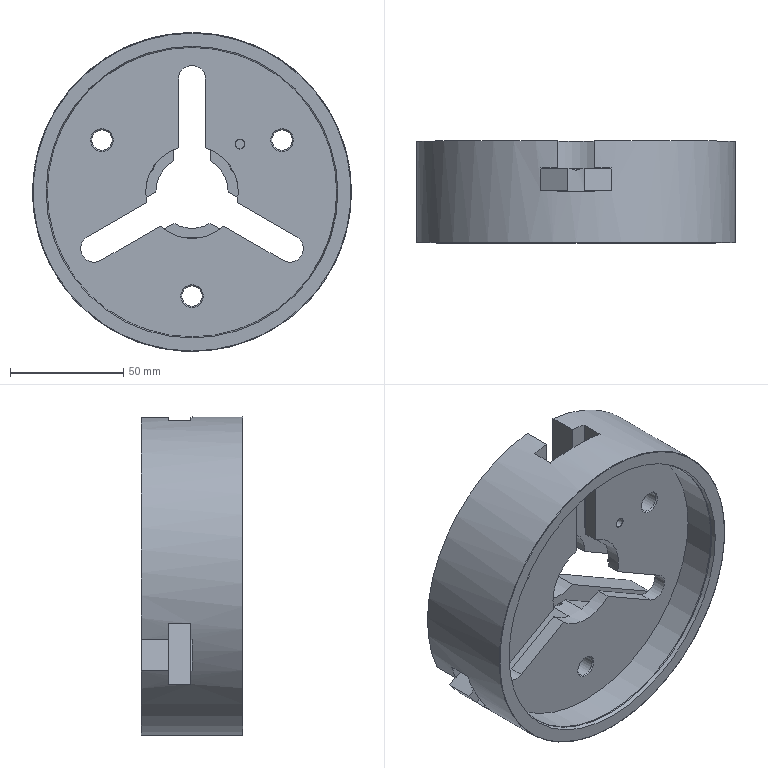NC program | NX | posted with a generic post | part box 141 x 45 x 141 mm
Whole program:
N10 G17 G21 G94 G90
(PLANAR_MILL , TOOL : D14)
N12 T05 M6
N14 G54
N16 G17 G0 G90 X0. Y89. S3600 M3
N18 G43 Z100. H5
N20 Z-1.
N22 G94 G1 Z-2. F3600.
N24 Y75.
N26 X0.9
N28 Y7.1
N30 X-0.9
N32 Y75.
N34 X0.
N36 Y89.
N38 Z-1.
N40 G0 Z0.3
N42 Z-3.
N44 G1 Z-4.
N46 Y75.
N48 X0.9
N50 Y7.1
N52 X-0.9
N54 Y75.
N56 X0.
N58 Y89.
N60 Z-3.
N62 G0 Z-1.7
N64 Z-5.
N66 G1 Z-6.
N68 Y75.
N70 X0.9
N72 Y7.1
N74 X-0.9
N76 Y75.
N78 X0.
N80 Y89.
N82 Z-5.
N84 G0 Z-3.7
N86 Z-7.
N88 G1 Z-8.
N90 Y75.
N92 X0.9
N94 Y7.1
N96 X-0.9
N98 Y75.
N100 X0.
N102 Y89.
N104 Z-7.
N106 G0 Z-5.7
N108 Z-9.
N110 G1 Z-10.
N112 Y75.
N114 X0.9
N116 Y7.1
N118 X-0.9
N120 Y75.
N122 X0.
N124 Y89.
N126 Z-9.
N128 G0 Z-7.7
N130 Z-11.
N132 G1 Z-12.
N134 Y75.
N136 X0.9
N138 Y7.1
N140 X-0.9
N142 Y75.
N144 X0.
N146 Y89.
N148 Z-11.
N150 G0 Z-9.7
N152 Z-13.
N154 G1 Z-14.
N156 Y75.
N158 X0.9
N160 Y7.1
N162 X-0.9
N164 Y75.
N166 X0.
N168 Y89.
N170 Z-13.
N172 G0 Z-11.7
N174 Z-15.
N176 G1 Z-16.
N178 Y75.
N180 X0.9
N182 Y7.1
N184 X-0.9
N186 Y75.
N188 X0.
N190 Y89.
N192 Z-15.
N194 G0 Z-13.7
N196 Z-17.
N198 G1 Z-18.
N200 Y75.
N202 X0.9
N204 Y7.1
N206 X-0.9
N208 Y75.
N210 X0.
N212 Y89.
N214 Z-17.
N216 G0 Z-15.7
N218 Z-19.
N220 G1 Z-20.
N222 Y75.
N224 X0.9
N226 Y7.1
N228 X-0.9
N230 Y75.
N232 X0.
N234 Y89.
N236 Z-19.
N238 G0 Z-17.7
N240 Z-21.
N242 G1 Z-22.
N244 Y75.
N246 X0.9
N248 Y7.1
N250 X-0.9
N252 Y75.
N254 X0.
N256 Y89.
N258 Z-21.
N260 G0 Z-19.7
N262 Z-21.4
N264 G1 Z-22.4
N266 Y75.
N268 X0.9
N270 Y7.1
N272 X-0.9
N274 Y75.
N276 X0.
N278 Y89.
N280 Z-21.4
N282 G0 Z100.
(PLANAR_MILL_COPY , TOOL : D14)
N284 X-77.076 Y-44.5
N286 Z-1.
N288 G1 Z-2.
N290 X-64.952 Y-37.5
N292 X-65.402 Y-36.721
N294 X-6.599 Y-2.771
N296 X-5.699 Y-4.329
N298 X-64.502 Y-38.279
N300 X-64.952 Y-37.5
N302 X-77.076 Y-44.5
N304 Z-1.
N306 G0 Z0.3
N308 Z-3.
N310 G1 Z-4.
N312 X-64.952 Y-37.5
N314 X-65.402 Y-36.721
N316 X-6.599 Y-2.771
N318 X-5.699 Y-4.329
N320 X-64.502 Y-38.279
N322 X-64.952 Y-37.5
N324 X-77.076 Y-44.5
N326 Z-3.
N328 G0 Z-1.7
N330 Z-5.
N332 G1 Z-6.
N334 X-64.952 Y-37.5
N336 X-65.402 Y-36.721
N338 X-6.599 Y-2.771
N340 X-5.699 Y-4.329
N342 X-64.502 Y-38.279
N344 X-64.952 Y-37.5
N346 X-77.076 Y-44.5
N348 Z-5.
N350 G0 Z-3.7
N352 Z-7.
N354 G1 Z-8.
N356 X-64.952 Y-37.5
N358 X-65.402 Y-36.721
N360 X-6.599 Y-2.771
N362 X-5.699 Y-4.329
N364 X-64.502 Y-38.279
N366 X-64.952 Y-37.5
N368 X-77.076 Y-44.5
N370 Z-7.
N372 G0 Z-5.7
N374 Z-9.
N376 G1 Z-10.
N378 X-64.952 Y-37.5
N380 X-65.402 Y-36.721
N382 X-6.599 Y-2.771
N384 X-5.699 Y-4.329
N386 X-64.502 Y-38.279
N388 X-64.952 Y-37.5
N390 X-77.076 Y-44.5
N392 Z-9.
N394 G0 Z-7.7
N396 Z-11.
N398 G1 Z-12.
N400 X-64.952 Y-37.5
N402 X-65.402 Y-36.721
N404 X-6.599 Y-2.771
N406 X-5.699 Y-4.329
N408 X-64.502 Y-38.279
N410 X-64.952 Y-37.5
N412 X-77.076 Y-44.5
N414 Z-11.
N416 G0 Z-9.7
N418 Z-13.
N420 G1 Z-14.
N422 X-64.952 Y-37.5
N424 X-65.402 Y-36.721
N426 X-6.599 Y-2.771
N428 X-5.699 Y-4.329
N430 X-64.502 Y-38.279
N432 X-64.952 Y-37.5
N434 X-77.076 Y-44.5
N436 Z-13.
N438 G0 Z-11.7
N440 Z-15.
N442 G1 Z-16.
N444 X-64.952 Y-37.5
N446 X-65.402 Y-36.721
N448 X-6.599 Y-2.771
N450 X-5.699 Y-4.329
N452 X-64.502 Y-38.279
N454 X-64.952 Y-37.5
N456 X-77.076 Y-44.5
N458 Z-15.
N460 G0 Z-13.7
N462 Z-17.
N464 G1 Z-18.
N466 X-64.952 Y-37.5
N468 X-65.402 Y-36.721
N470 X-6.599 Y-2.771
N472 X-5.699 Y-4.329
N474 X-64.502 Y-38.279
N476 X-64.952 Y-37.5
N478 X-77.076 Y-44.5
N480 Z-17.
N482 G0 Z-15.7
N484 Z-19.
N486 G1 Z-20.
N488 X-64.952 Y-37.5
N490 X-65.402 Y-36.721
N492 X-6.599 Y-2.771
N494 X-5.699 Y-4.329
N496 X-64.502 Y-38.279
N498 X-64.952 Y-37.5
N500 X-77.076 Y-44.5
N502 Z-19.
N504 G0 Z-17.7
N506 Z-21.
N508 G1 Z-22.
N510 X-64.952 Y-37.5
N512 X-65.402 Y-36.721
N514 X-6.599 Y-2.771
N516 X-5.699 Y-4.329
N518 X-64.502 Y-38.279
N520 X-64.952 Y-37.5
N522 X-77.076 Y-44.5
N524 Z-21.
N526 G0 Z-19.7
N528 Z-21.4
N530 G1 Z-22.4
N532 X-64.952 Y-37.5
N534 X-65.402 Y-36.721
N536 X-6.599 Y-2.771
N538 X-5.699 Y-4.329
N540 X-64.502 Y-38.279
N542 X-64.952 Y-37.5
N544 X-77.076 Y-44.5
N546 Z-21.4
N548 G0 Z100.
(PLANAR_MILL_COPY_1 , TOOL : D14)
N550 X77.076
N552 Z-1.
N554 G1 Z-2.
N556 X64.952 Y-37.5
N558 X64.502 Y-38.279
N560 X5.699 Y-4.329
N562 X6.599 Y-2.771
N564 X65.402 Y-36.721
N566 X64.952 Y-37.5
N568 X77.076 Y-44.5
N570 Z-1.
N572 G0 Z0.3
N574 Z-3.
N576 G1 Z-4.
N578 X64.952 Y-37.5
N580 X64.502 Y-38.279
N582 X5.699 Y-4.329
N584 X6.599 Y-2.771
N586 X65.402 Y-36.721
N588 X64.952 Y-37.5
N590 X77.076 Y-44.5
N592 Z-3.
N594 G0 Z-1.7
N596 Z-5.
N598 G1 Z-6.
N600 X64.952 Y-37.5
N602 X64.502 Y-38.279
N604 X5.699 Y-4.329
N606 X6.599 Y-2.771
N608 X65.402 Y-36.721
N610 X64.952 Y-37.5
N612 X77.076 Y-44.5
N614 Z-5.
N616 G0 Z-3.7
N618 Z-7.
N620 G1 Z-8.
N622 X64.952 Y-37.5
N624 X64.502 Y-38.279
N626 X5.699 Y-4.329
N628 X6.599 Y-2.771
N630 X65.402 Y-36.721
N632 X64.952 Y-37.5
N634 X77.076 Y-44.5
N636 Z-7.
N638 G0 Z-5.7
N640 Z-9.
N642 G1 Z-10.
N644 X64.952 Y-37.5
N646 X64.502 Y-38.279
N648 X5.699 Y-4.329
N650 X6.599 Y-2.771
N652 X65.402 Y-36.721
N654 X64.952 Y-37.5
N656 X77.076 Y-44.5
N658 Z-9.
N660 G0 Z-7.7
N662 Z-11.
N664 G1 Z-12.
N666 X64.952 Y-37.5
N668 X64.502 Y-38.279
N670 X5.699 Y-4.329
N672 X6.599 Y-2.771
N674 X65.402 Y-36.721
N676 X64.952 Y-37.5
N678 X77.076 Y-44.5
N680 Z-11.
N682 G0 Z-9.7
N684 Z-13.
N686 G1 Z-14.
N688 X64.952 Y-37.5
N690 X64.502 Y-38.279
N692 X5.699 Y-4.329
N694 X6.599 Y-2.771
N696 X65.402 Y-36.721
N698 X64.952 Y-37.5
N700 X77.076 Y-44.5
N702 Z-13.
N704 G0 Z-11.7
N706 Z-15.
N708 G1 Z-16.
N710 X64.952 Y-37.5
N712 X64.502 Y-38.279
N714 X5.699 Y-4.329
N716 X6.599 Y-2.771
N718 X65.402 Y-36.721
N720 X64.952 Y-37.5
N722 X77.076 Y-44.5
N724 Z-15.
N726 G0 Z-13.7
N728 Z-17.
N730 G1 Z-18.
N732 X64.952 Y-37.5
N734 X64.502 Y-38.279
N736 X5.699 Y-4.329
N738 X6.599 Y-2.771
N740 X65.402 Y-36.721
N742 X64.952 Y-37.5
N744 X77.076 Y-44.5
N746 Z-17.
N748 G0 Z-15.7
N750 Z-19.
N752 G1 Z-20.
N754 X64.952 Y-37.5
N756 X64.502 Y-38.279
N758 X5.699 Y-4.329
N760 X6.599 Y-2.771
N762 X65.402 Y-36.721
N764 X64.952 Y-37.5
N766 X77.076 Y-44.5
N768 Z-19.
N770 G0 Z-17.7
N772 Z-21.
N774 G1 Z-22.
N776 X64.952 Y-37.5
N778 X64.502 Y-38.279
N780 X5.699 Y-4.329
N782 X6.599 Y-2.771
N784 X65.402 Y-36.721
N786 X64.952 Y-37.5
N788 X77.076 Y-44.5
N790 Z-21.
N792 G0 Z-19.7
N794 Z-21.4
N796 G1 Z-22.4
N798 X64.952 Y-37.5
N800 X64.502 Y-38.279
N802 X5.699 Y-4.329
N804 X6.599 Y-2.771
N806 X65.402 Y-36.721
N808 X64.952 Y-37.5
N810 X77.076 Y-44.5
N812 Z-21.4
N814 G0 Z100.
N816 M5
N818 M2